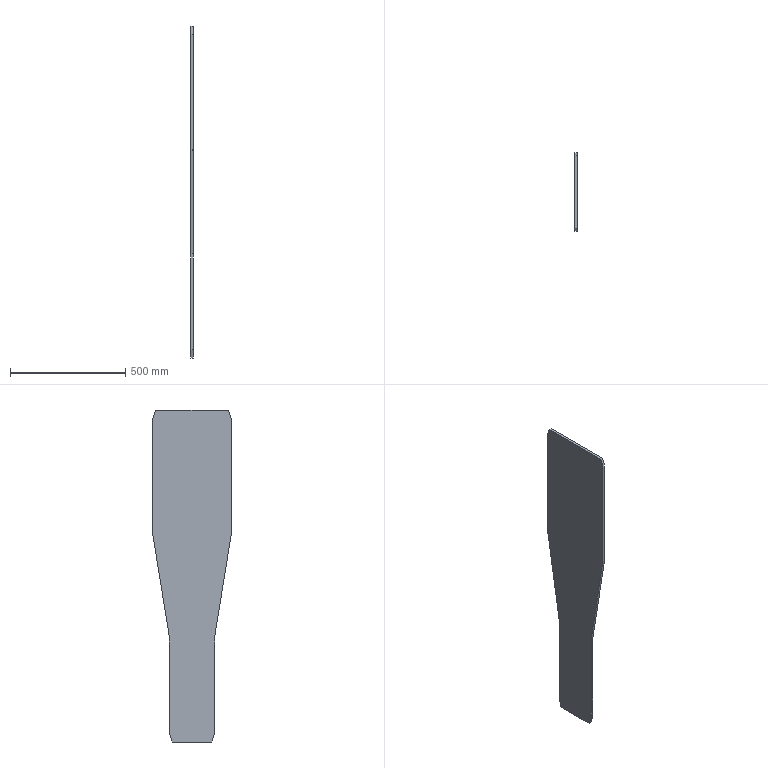Part | SolidWorks | features Extrusion 1 | 1 solid | 18 faces | box 10 x 340 x 1438 mm | volume 3900020 mm3 | plane 14 | cylinder 4 | commonest cylinder face diameters 20 x4
STEP:
#1=CARTESIAN_POINT('',(0.,85.5,-1438.));
#2=VERTEX_POINT('',#1);
#3=CARTESIAN_POINT('',(0.,97.5,-1403.));
#4=VERTEX_POINT('',#3);
#5=CARTESIAN_POINT('',(0.,85.5,-1438.));
#6=DIRECTION('',(0.,0.3243,0.9459));
#7=VECTOR('',#6,1000.);
#8=LINE('',#5,#7);
#9=EDGE_CURVE('',#2,#4,#8,.T.);
#10=ORIENTED_EDGE('',*,*,#9,.T.);
#11=CARTESIAN_POINT('',(10.,97.5,-1403.));
#12=VERTEX_POINT('',#11);
#13=CARTESIAN_POINT('',(10.,97.5,-1403.));
#14=DIRECTION('',(-1.,0.,0.));
#15=VECTOR('',#14,1000.);
#16=LINE('',#13,#15);
#17=EDGE_CURVE('',#12,#4,#16,.T.);
#18=ORIENTED_EDGE('',*,*,#17,.F.);
#19=CARTESIAN_POINT('',(10.,85.5,-1438.));
#20=VERTEX_POINT('',#19);
#21=CARTESIAN_POINT('',(10.,85.5,-1438.));
#22=DIRECTION('',(0.,0.3243,0.9459));
#23=VECTOR('',#22,1000.);
#24=LINE('',#21,#23);
#25=EDGE_CURVE('',#20,#12,#24,.T.);
#26=ORIENTED_EDGE('',*,*,#25,.F.);
#27=CARTESIAN_POINT('',(10.,85.5,-1438.));
#28=DIRECTION('',(-1.,0.,0.));
#29=VECTOR('',#28,1000.);
#30=LINE('',#27,#29);
#31=EDGE_CURVE('',#20,#2,#30,.T.);
#32=ORIENTED_EDGE('',*,*,#31,.T.);
#33=EDGE_LOOP('',(#10,#18,#26,#32));
#34=FACE_OUTER_BOUND('',#33,.T.);
#35=CARTESIAN_POINT('',(10.,85.5,-1438.));
#36=DIRECTION('',(0.,-0.9459,0.3243));
#37=DIRECTION('',(0.,-0.3243,-0.9459));
#38=AXIS2_PLACEMENT_3D('',#35,#36,#37);
#39=PLANE('',#38);
#40=ADVANCED_FACE('',(#34),#39,.F.);
#41=CARTESIAN_POINT('',(0.,97.5,-987.4));
#42=VERTEX_POINT('',#41);
#43=CARTESIAN_POINT('',(0.,97.5,-987.4));
#44=DIRECTION('',(0.,0.,1.));
#45=VECTOR('',#44,1000.);
#46=LINE('',#43,#45);
#47=EDGE_CURVE('',#4,#42,#46,.T.);
#48=ORIENTED_EDGE('',*,*,#47,.T.);
#49=CARTESIAN_POINT('',(10.,97.5,-987.4));
#50=VERTEX_POINT('',#49);
#51=CARTESIAN_POINT('',(10.,97.5,-987.4));
#52=DIRECTION('',(-1.,0.,0.));
#53=VECTOR('',#52,1000.);
#54=LINE('',#51,#53);
#55=EDGE_CURVE('',#50,#42,#54,.T.);
#56=ORIENTED_EDGE('',*,*,#55,.F.);
#57=CARTESIAN_POINT('',(10.,97.5,-987.4));
#58=DIRECTION('',(0.,0.,1.));
#59=VECTOR('',#58,1000.);
#60=LINE('',#57,#59);
#61=EDGE_CURVE('',#12,#50,#60,.T.);
#62=ORIENTED_EDGE('',*,*,#61,.F.);
#63=ORIENTED_EDGE('',*,*,#17,.T.);
#64=EDGE_LOOP('',(#48,#56,#62,#63));
#65=FACE_OUTER_BOUND('',#64,.T.);
#66=CARTESIAN_POINT('',(10.,97.5,-987.4));
#67=DIRECTION('',(0.,-1.,0.));
#68=DIRECTION('',(0.,0.,-1.));
#69=AXIS2_PLACEMENT_3D('',#66,#67,#68);
#70=PLANE('',#69);
#71=ADVANCED_FACE('',(#65),#70,.F.);
#72=CARTESIAN_POINT('',(0.,97.627,-985.81));
#73=VERTEX_POINT('',#72);
#74=CARTESIAN_POINT('',(0.,107.5,-987.4));
#75=DIRECTION('',(-1.,0.,0.));
#76=DIRECTION('',(0.,0.,1.));
#77=AXIS2_PLACEMENT_3D('',#74,#75,#76);
#78=CIRCLE('',#77,10.);
#79=EDGE_CURVE('',#42,#73,#78,.T.);
#80=ORIENTED_EDGE('',*,*,#79,.T.);
#81=CARTESIAN_POINT('',(10.,97.627,-985.81));
#82=VERTEX_POINT('',#81);
#83=CARTESIAN_POINT('',(10.,97.627,-985.81));
#84=DIRECTION('',(-1.,0.,0.));
#85=VECTOR('',#84,1000.);
#86=LINE('',#83,#85);
#87=EDGE_CURVE('',#82,#73,#86,.T.);
#88=ORIENTED_EDGE('',*,*,#87,.F.);
#89=CARTESIAN_POINT('',(10.,107.5,-987.4));
#90=DIRECTION('',(-1.,0.,0.));
#91=DIRECTION('',(0.,0.,1.));
#92=AXIS2_PLACEMENT_3D('',#89,#90,#91);
#93=CIRCLE('',#92,10.);
#94=EDGE_CURVE('',#50,#82,#93,.T.);
#95=ORIENTED_EDGE('',*,*,#94,.F.);
#96=ORIENTED_EDGE('',*,*,#55,.T.);
#97=EDGE_LOOP('',(#80,#88,#95,#96));
#98=FACE_OUTER_BOUND('',#97,.T.);
#99=CARTESIAN_POINT('',(10.,107.5,-987.4));
#100=DIRECTION('',(-1.,0.,0.));
#101=DIRECTION('',(0.,0.,1.));
#102=AXIS2_PLACEMENT_3D('',#99,#100,#101);
#103=CYLINDRICAL_SURFACE('',#102,10.);
#104=ADVANCED_FACE('',(#98),#103,.F.);
#105=CARTESIAN_POINT('',(0.,169.873,-537.39));
#106=VERTEX_POINT('',#105);
#107=CARTESIAN_POINT('',(0.,169.873,-537.39));
#108=DIRECTION('',(0.,0.1591,0.9873));
#109=VECTOR('',#108,1000.);
#110=LINE('',#107,#109);
#111=EDGE_CURVE('',#73,#106,#110,.T.);
#112=ORIENTED_EDGE('',*,*,#111,.T.);
#113=CARTESIAN_POINT('',(10.,169.873,-537.39));
#114=VERTEX_POINT('',#113);
#115=CARTESIAN_POINT('',(10.,169.873,-537.39));
#116=DIRECTION('',(-1.,0.,0.));
#117=VECTOR('',#116,1000.);
#118=LINE('',#115,#117);
#119=EDGE_CURVE('',#114,#106,#118,.T.);
#120=ORIENTED_EDGE('',*,*,#119,.F.);
#121=CARTESIAN_POINT('',(10.,169.873,-537.39));
#122=DIRECTION('',(0.,0.1591,0.9873));
#123=VECTOR('',#122,1000.);
#124=LINE('',#121,#123);
#125=EDGE_CURVE('',#82,#114,#124,.T.);
#126=ORIENTED_EDGE('',*,*,#125,.F.);
#127=ORIENTED_EDGE('',*,*,#87,.T.);
#128=EDGE_LOOP('',(#112,#120,#126,#127));
#129=FACE_OUTER_BOUND('',#128,.T.);
#130=CARTESIAN_POINT('',(10.,169.873,-537.39));
#131=DIRECTION('',(0.,-0.9873,0.1591));
#132=DIRECTION('',(0.,-0.1591,-0.9873));
#133=AXIS2_PLACEMENT_3D('',#130,#131,#132);
#134=PLANE('',#133);
#135=ADVANCED_FACE('',(#129),#134,.F.);
#136=CARTESIAN_POINT('',(0.,170.,-535.8));
#137=VERTEX_POINT('',#136);
#138=CARTESIAN_POINT('',(0.,160.,-535.8));
#139=DIRECTION('',(1.,0.,0.));
#140=DIRECTION('',(0.,0.,-1.));
#141=AXIS2_PLACEMENT_3D('',#138,#139,#140);
#142=CIRCLE('',#141,10.);
#143=EDGE_CURVE('',#106,#137,#142,.T.);
#144=ORIENTED_EDGE('',*,*,#143,.T.);
#145=CARTESIAN_POINT('',(10.,170.,-535.8));
#146=VERTEX_POINT('',#145);
#147=CARTESIAN_POINT('',(10.,170.,-535.8));
#148=DIRECTION('',(-1.,0.,0.));
#149=VECTOR('',#148,1000.);
#150=LINE('',#147,#149);
#151=EDGE_CURVE('',#146,#137,#150,.T.);
#152=ORIENTED_EDGE('',*,*,#151,.F.);
#153=CARTESIAN_POINT('',(10.,160.,-535.8));
#154=DIRECTION('',(1.,0.,0.));
#155=DIRECTION('',(0.,0.,-1.));
#156=AXIS2_PLACEMENT_3D('',#153,#154,#155);
#157=CIRCLE('',#156,10.);
#158=EDGE_CURVE('',#114,#146,#157,.T.);
#159=ORIENTED_EDGE('',*,*,#158,.F.);
#160=ORIENTED_EDGE('',*,*,#119,.T.);
#161=EDGE_LOOP('',(#144,#152,#159,#160));
#162=FACE_OUTER_BOUND('',#161,.T.);
#163=CARTESIAN_POINT('',(10.,160.,-535.8));
#164=DIRECTION('',(-1.,0.,0.));
#165=DIRECTION('',(0.,0.,1.));
#166=AXIS2_PLACEMENT_3D('',#163,#164,#165);
#167=CYLINDRICAL_SURFACE('',#166,10.);
#168=ADVANCED_FACE('',(#162),#167,.T.);
#169=CARTESIAN_POINT('',(0.,170.,-35.));
#170=VERTEX_POINT('',#169);
#171=CARTESIAN_POINT('',(0.,170.,-35.));
#172=DIRECTION('',(0.,0.,1.));
#173=VECTOR('',#172,1000.);
#174=LINE('',#171,#173);
#175=EDGE_CURVE('',#137,#170,#174,.T.);
#176=ORIENTED_EDGE('',*,*,#175,.T.);
#177=CARTESIAN_POINT('',(10.,170.,-35.));
#178=VERTEX_POINT('',#177);
#179=CARTESIAN_POINT('',(10.,170.,-35.));
#180=DIRECTION('',(-1.,0.,0.));
#181=VECTOR('',#180,1000.);
#182=LINE('',#179,#181);
#183=EDGE_CURVE('',#178,#170,#182,.T.);
#184=ORIENTED_EDGE('',*,*,#183,.F.);
#185=CARTESIAN_POINT('',(10.,170.,-35.));
#186=DIRECTION('',(0.,0.,1.));
#187=VECTOR('',#186,1000.);
#188=LINE('',#185,#187);
#189=EDGE_CURVE('',#146,#178,#188,.T.);
#190=ORIENTED_EDGE('',*,*,#189,.F.);
#191=ORIENTED_EDGE('',*,*,#151,.T.);
#192=EDGE_LOOP('',(#176,#184,#190,#191));
#193=FACE_OUTER_BOUND('',#192,.T.);
#194=CARTESIAN_POINT('',(10.,170.,-35.));
#195=DIRECTION('',(0.,-1.,0.));
#196=DIRECTION('',(0.,0.,-1.));
#197=AXIS2_PLACEMENT_3D('',#194,#195,#196);
#198=PLANE('',#197);
#199=ADVANCED_FACE('',(#193),#198,.F.);
#200=CARTESIAN_POINT('',(0.,158.,0.));
#201=VERTEX_POINT('',#200);
#202=CARTESIAN_POINT('',(0.,158.,0.));
#203=DIRECTION('',(0.,-0.3243,0.9459));
#204=VECTOR('',#203,1000.);
#205=LINE('',#202,#204);
#206=EDGE_CURVE('',#170,#201,#205,.T.);
#207=ORIENTED_EDGE('',*,*,#206,.T.);
#208=CARTESIAN_POINT('',(10.,158.,0.));
#209=VERTEX_POINT('',#208);
#210=CARTESIAN_POINT('',(10.,158.,0.));
#211=DIRECTION('',(-1.,0.,0.));
#212=VECTOR('',#211,1000.);
#213=LINE('',#210,#212);
#214=EDGE_CURVE('',#209,#201,#213,.T.);
#215=ORIENTED_EDGE('',*,*,#214,.F.);
#216=CARTESIAN_POINT('',(10.,158.,0.));
#217=DIRECTION('',(0.,-0.3243,0.9459));
#218=VECTOR('',#217,1000.);
#219=LINE('',#216,#218);
#220=EDGE_CURVE('',#178,#209,#219,.T.);
#221=ORIENTED_EDGE('',*,*,#220,.F.);
#222=ORIENTED_EDGE('',*,*,#183,.T.);
#223=EDGE_LOOP('',(#207,#215,#221,#222));
#224=FACE_OUTER_BOUND('',#223,.T.);
#225=CARTESIAN_POINT('',(10.,158.,0.));
#226=DIRECTION('',(0.,-0.9459,-0.3243));
#227=DIRECTION('',(0.,0.3243,-0.9459));
#228=AXIS2_PLACEMENT_3D('',#225,#226,#227);
#229=PLANE('',#228);
#230=ADVANCED_FACE('',(#224),#229,.F.);
#231=CARTESIAN_POINT('',(0.,-158.,0.));
#232=VERTEX_POINT('',#231);
#233=CARTESIAN_POINT('',(0.,-158.,0.));
#234=DIRECTION('',(0.,-1.,0.));
#235=VECTOR('',#234,1000.);
#236=LINE('',#233,#235);
#237=EDGE_CURVE('',#201,#232,#236,.T.);
#238=ORIENTED_EDGE('',*,*,#237,.T.);
#239=CARTESIAN_POINT('',(10.,-158.,0.));
#240=VERTEX_POINT('',#239);
#241=CARTESIAN_POINT('',(10.,-158.,0.));
#242=DIRECTION('',(-1.,0.,0.));
#243=VECTOR('',#242,1000.);
#244=LINE('',#241,#243);
#245=EDGE_CURVE('',#240,#232,#244,.T.);
#246=ORIENTED_EDGE('',*,*,#245,.F.);
#247=CARTESIAN_POINT('',(10.,-158.,0.));
#248=DIRECTION('',(0.,-1.,0.));
#249=VECTOR('',#248,1000.);
#250=LINE('',#247,#249);
#251=EDGE_CURVE('',#209,#240,#250,.T.);
#252=ORIENTED_EDGE('',*,*,#251,.F.);
#253=ORIENTED_EDGE('',*,*,#214,.T.);
#254=EDGE_LOOP('',(#238,#246,#252,#253));
#255=FACE_OUTER_BOUND('',#254,.T.);
#256=CARTESIAN_POINT('',(10.,-158.,0.));
#257=DIRECTION('',(0.,0.,-1.));
#258=DIRECTION('',(-1.,0.,0.));
#259=AXIS2_PLACEMENT_3D('',#256,#257,#258);
#260=PLANE('',#259);
#261=ADVANCED_FACE('',(#255),#260,.F.);
#262=CARTESIAN_POINT('',(0.,-170.,-35.));
#263=VERTEX_POINT('',#262);
#264=CARTESIAN_POINT('',(0.,-158.,0.));
#265=DIRECTION('',(0.,-0.3243,-0.9459));
#266=VECTOR('',#265,1000.);
#267=LINE('',#264,#266);
#268=EDGE_CURVE('',#232,#263,#267,.T.);
#269=ORIENTED_EDGE('',*,*,#268,.T.);
#270=CARTESIAN_POINT('',(10.,-170.,-35.));
#271=VERTEX_POINT('',#270);
#272=CARTESIAN_POINT('',(10.,-170.,-35.));
#273=DIRECTION('',(-1.,0.,0.));
#274=VECTOR('',#273,1000.);
#275=LINE('',#272,#274);
#276=EDGE_CURVE('',#271,#263,#275,.T.);
#277=ORIENTED_EDGE('',*,*,#276,.F.);
#278=CARTESIAN_POINT('',(10.,-158.,0.));
#279=DIRECTION('',(0.,-0.3243,-0.9459));
#280=VECTOR('',#279,1000.);
#281=LINE('',#278,#280);
#282=EDGE_CURVE('',#240,#271,#281,.T.);
#283=ORIENTED_EDGE('',*,*,#282,.F.);
#284=ORIENTED_EDGE('',*,*,#245,.T.);
#285=EDGE_LOOP('',(#269,#277,#283,#284));
#286=FACE_OUTER_BOUND('',#285,.T.);
#287=CARTESIAN_POINT('',(10.,-158.,0.));
#288=DIRECTION('',(0.,0.9459,-0.3243));
#289=DIRECTION('',(0.,0.3243,0.9459));
#290=AXIS2_PLACEMENT_3D('',#287,#288,#289);
#291=PLANE('',#290);
#292=ADVANCED_FACE('',(#286),#291,.F.);
#293=CARTESIAN_POINT('',(0.,-170.,-535.8));
#294=VERTEX_POINT('',#293);
#295=CARTESIAN_POINT('',(0.,-170.,-35.));
#296=DIRECTION('',(0.,0.,-1.));
#297=VECTOR('',#296,1000.);
#298=LINE('',#295,#297);
#299=EDGE_CURVE('',#263,#294,#298,.T.);
#300=ORIENTED_EDGE('',*,*,#299,.T.);
#301=CARTESIAN_POINT('',(10.,-170.,-535.8));
#302=VERTEX_POINT('',#301);
#303=CARTESIAN_POINT('',(10.,-170.,-535.8));
#304=DIRECTION('',(-1.,0.,0.));
#305=VECTOR('',#304,1000.);
#306=LINE('',#303,#305);
#307=EDGE_CURVE('',#302,#294,#306,.T.);
#308=ORIENTED_EDGE('',*,*,#307,.F.);
#309=CARTESIAN_POINT('',(10.,-170.,-35.));
#310=DIRECTION('',(0.,0.,-1.));
#311=VECTOR('',#310,1000.);
#312=LINE('',#309,#311);
#313=EDGE_CURVE('',#271,#302,#312,.T.);
#314=ORIENTED_EDGE('',*,*,#313,.F.);
#315=ORIENTED_EDGE('',*,*,#276,.T.);
#316=EDGE_LOOP('',(#300,#308,#314,#315));
#317=FACE_OUTER_BOUND('',#316,.T.);
#318=CARTESIAN_POINT('',(10.,-170.,-35.));
#319=DIRECTION('',(0.,1.,0.));
#320=DIRECTION('',(0.,0.,1.));
#321=AXIS2_PLACEMENT_3D('',#318,#319,#320);
#322=PLANE('',#321);
#323=ADVANCED_FACE('',(#317),#322,.F.);
#324=CARTESIAN_POINT('',(0.,-169.873,-537.39));
#325=VERTEX_POINT('',#324);
#326=CARTESIAN_POINT('',(0.,-160.,-535.8));
#327=DIRECTION('',(1.,0.,0.));
#328=DIRECTION('',(0.,0.,1.));
#329=AXIS2_PLACEMENT_3D('',#326,#327,#328);
#330=CIRCLE('',#329,10.);
#331=EDGE_CURVE('',#294,#325,#330,.T.);
#332=ORIENTED_EDGE('',*,*,#331,.T.);
#333=CARTESIAN_POINT('',(10.,-169.873,-537.39));
#334=VERTEX_POINT('',#333);
#335=CARTESIAN_POINT('',(10.,-169.873,-537.39));
#336=DIRECTION('',(-1.,0.,0.));
#337=VECTOR('',#336,1000.);
#338=LINE('',#335,#337);
#339=EDGE_CURVE('',#334,#325,#338,.T.);
#340=ORIENTED_EDGE('',*,*,#339,.F.);
#341=CARTESIAN_POINT('',(10.,-160.,-535.8));
#342=DIRECTION('',(1.,0.,0.));
#343=DIRECTION('',(0.,0.,1.));
#344=AXIS2_PLACEMENT_3D('',#341,#342,#343);
#345=CIRCLE('',#344,10.);
#346=EDGE_CURVE('',#302,#334,#345,.T.);
#347=ORIENTED_EDGE('',*,*,#346,.F.);
#348=ORIENTED_EDGE('',*,*,#307,.T.);
#349=EDGE_LOOP('',(#332,#340,#347,#348));
#350=FACE_OUTER_BOUND('',#349,.T.);
#351=CARTESIAN_POINT('',(10.,-160.,-535.8));
#352=DIRECTION('',(-1.,0.,0.));
#353=DIRECTION('',(0.,0.,1.));
#354=AXIS2_PLACEMENT_3D('',#351,#352,#353);
#355=CYLINDRICAL_SURFACE('',#354,10.);
#356=ADVANCED_FACE('',(#350),#355,.T.);
#357=CARTESIAN_POINT('',(0.,-97.627,-985.81));
#358=VERTEX_POINT('',#357);
#359=CARTESIAN_POINT('',(0.,-169.873,-537.39));
#360=DIRECTION('',(0.,0.1591,-0.9873));
#361=VECTOR('',#360,1000.);
#362=LINE('',#359,#361);
#363=EDGE_CURVE('',#325,#358,#362,.T.);
#364=ORIENTED_EDGE('',*,*,#363,.T.);
#365=CARTESIAN_POINT('',(10.,-97.627,-985.81));
#366=VERTEX_POINT('',#365);
#367=CARTESIAN_POINT('',(10.,-97.627,-985.81));
#368=DIRECTION('',(-1.,0.,0.));
#369=VECTOR('',#368,1000.);
#370=LINE('',#367,#369);
#371=EDGE_CURVE('',#366,#358,#370,.T.);
#372=ORIENTED_EDGE('',*,*,#371,.F.);
#373=CARTESIAN_POINT('',(10.,-169.873,-537.39));
#374=DIRECTION('',(0.,0.1591,-0.9873));
#375=VECTOR('',#374,1000.);
#376=LINE('',#373,#375);
#377=EDGE_CURVE('',#334,#366,#376,.T.);
#378=ORIENTED_EDGE('',*,*,#377,.F.);
#379=ORIENTED_EDGE('',*,*,#339,.T.);
#380=EDGE_LOOP('',(#364,#372,#378,#379));
#381=FACE_OUTER_BOUND('',#380,.T.);
#382=CARTESIAN_POINT('',(10.,-169.873,-537.39));
#383=DIRECTION('',(0.,0.9873,0.1591));
#384=DIRECTION('',(0.,-0.1591,0.9873));
#385=AXIS2_PLACEMENT_3D('',#382,#383,#384);
#386=PLANE('',#385);
#387=ADVANCED_FACE('',(#381),#386,.F.);
#388=CARTESIAN_POINT('',(0.,-97.5,-987.4));
#389=VERTEX_POINT('',#388);
#390=CARTESIAN_POINT('',(0.,-107.5,-987.4));
#391=DIRECTION('',(-1.,0.,0.));
#392=DIRECTION('',(0.,0.,-1.));
#393=AXIS2_PLACEMENT_3D('',#390,#391,#392);
#394=CIRCLE('',#393,10.);
#395=EDGE_CURVE('',#358,#389,#394,.T.);
#396=ORIENTED_EDGE('',*,*,#395,.T.);
#397=CARTESIAN_POINT('',(10.,-97.5,-987.4));
#398=VERTEX_POINT('',#397);
#399=CARTESIAN_POINT('',(10.,-97.5,-987.4));
#400=DIRECTION('',(-1.,0.,0.));
#401=VECTOR('',#400,1000.);
#402=LINE('',#399,#401);
#403=EDGE_CURVE('',#398,#389,#402,.T.);
#404=ORIENTED_EDGE('',*,*,#403,.F.);
#405=CARTESIAN_POINT('',(10.,-107.5,-987.4));
#406=DIRECTION('',(-1.,0.,0.));
#407=DIRECTION('',(0.,0.,-1.));
#408=AXIS2_PLACEMENT_3D('',#405,#406,#407);
#409=CIRCLE('',#408,10.);
#410=EDGE_CURVE('',#366,#398,#409,.T.);
#411=ORIENTED_EDGE('',*,*,#410,.F.);
#412=ORIENTED_EDGE('',*,*,#371,.T.);
#413=EDGE_LOOP('',(#396,#404,#411,#412));
#414=FACE_OUTER_BOUND('',#413,.T.);
#415=CARTESIAN_POINT('',(10.,-107.5,-987.4));
#416=DIRECTION('',(-1.,0.,0.));
#417=DIRECTION('',(0.,0.,1.));
#418=AXIS2_PLACEMENT_3D('',#415,#416,#417);
#419=CYLINDRICAL_SURFACE('',#418,10.);
#420=ADVANCED_FACE('',(#414),#419,.F.);
#421=CARTESIAN_POINT('',(0.,-97.5,-1403.));
#422=VERTEX_POINT('',#421);
#423=CARTESIAN_POINT('',(0.,-97.5,-987.4));
#424=DIRECTION('',(0.,0.,-1.));
#425=VECTOR('',#424,1000.);
#426=LINE('',#423,#425);
#427=EDGE_CURVE('',#389,#422,#426,.T.);
#428=ORIENTED_EDGE('',*,*,#427,.T.);
#429=CARTESIAN_POINT('',(10.,-97.5,-1403.));
#430=VERTEX_POINT('',#429);
#431=CARTESIAN_POINT('',(10.,-97.5,-1403.));
#432=DIRECTION('',(-1.,0.,0.));
#433=VECTOR('',#432,1000.);
#434=LINE('',#431,#433);
#435=EDGE_CURVE('',#430,#422,#434,.T.);
#436=ORIENTED_EDGE('',*,*,#435,.F.);
#437=CARTESIAN_POINT('',(10.,-97.5,-987.4));
#438=DIRECTION('',(0.,0.,-1.));
#439=VECTOR('',#438,1000.);
#440=LINE('',#437,#439);
#441=EDGE_CURVE('',#398,#430,#440,.T.);
#442=ORIENTED_EDGE('',*,*,#441,.F.);
#443=ORIENTED_EDGE('',*,*,#403,.T.);
#444=EDGE_LOOP('',(#428,#436,#442,#443));
#445=FACE_OUTER_BOUND('',#444,.T.);
#446=CARTESIAN_POINT('',(10.,-97.5,-987.4));
#447=DIRECTION('',(0.,1.,0.));
#448=DIRECTION('',(0.,0.,1.));
#449=AXIS2_PLACEMENT_3D('',#446,#447,#448);
#450=PLANE('',#449);
#451=ADVANCED_FACE('',(#445),#450,.F.);
#452=CARTESIAN_POINT('',(0.,-85.5,-1438.));
#453=VERTEX_POINT('',#452);
#454=CARTESIAN_POINT('',(0.,-85.5,-1438.));
#455=DIRECTION('',(0.,0.3243,-0.9459));
#456=VECTOR('',#455,1000.);
#457=LINE('',#454,#456);
#458=EDGE_CURVE('',#422,#453,#457,.T.);
#459=ORIENTED_EDGE('',*,*,#458,.T.);
#460=CARTESIAN_POINT('',(10.,-85.5,-1438.));
#461=VERTEX_POINT('',#460);
#462=CARTESIAN_POINT('',(10.,-85.5,-1438.));
#463=DIRECTION('',(-1.,0.,0.));
#464=VECTOR('',#463,1000.);
#465=LINE('',#462,#464);
#466=EDGE_CURVE('',#461,#453,#465,.T.);
#467=ORIENTED_EDGE('',*,*,#466,.F.);
#468=CARTESIAN_POINT('',(10.,-85.5,-1438.));
#469=DIRECTION('',(0.,0.3243,-0.9459));
#470=VECTOR('',#469,1000.);
#471=LINE('',#468,#470);
#472=EDGE_CURVE('',#430,#461,#471,.T.);
#473=ORIENTED_EDGE('',*,*,#472,.F.);
#474=ORIENTED_EDGE('',*,*,#435,.T.);
#475=EDGE_LOOP('',(#459,#467,#473,#474));
#476=FACE_OUTER_BOUND('',#475,.T.);
#477=CARTESIAN_POINT('',(10.,-85.5,-1438.));
#478=DIRECTION('',(0.,0.9459,0.3243));
#479=DIRECTION('',(0.,-0.3243,0.9459));
#480=AXIS2_PLACEMENT_3D('',#477,#478,#479);
#481=PLANE('',#480);
#482=ADVANCED_FACE('',(#476),#481,.F.);
#483=CARTESIAN_POINT('',(0.,85.5,-1438.));
#484=DIRECTION('',(0.,1.,0.));
#485=VECTOR('',#484,1000.);
#486=LINE('',#483,#485);
#487=EDGE_CURVE('',#453,#2,#486,.T.);
#488=ORIENTED_EDGE('',*,*,#487,.T.);
#489=ORIENTED_EDGE('',*,*,#31,.F.);
#490=CARTESIAN_POINT('',(10.,85.5,-1438.));
#491=DIRECTION('',(0.,1.,0.));
#492=VECTOR('',#491,1000.);
#493=LINE('',#490,#492);
#494=EDGE_CURVE('',#461,#20,#493,.T.);
#495=ORIENTED_EDGE('',*,*,#494,.F.);
#496=ORIENTED_EDGE('',*,*,#466,.T.);
#497=EDGE_LOOP('',(#488,#489,#495,#496));
#498=FACE_OUTER_BOUND('',#497,.T.);
#499=CARTESIAN_POINT('',(10.,85.5,-1438.));
#500=DIRECTION('',(0.,0.,1.));
#501=DIRECTION('',(1.,0.,0.));
#502=AXIS2_PLACEMENT_3D('',#499,#500,#501);
#503=PLANE('',#502);
#504=ADVANCED_FACE('',(#498),#503,.F.);
#505=ORIENTED_EDGE('',*,*,#25,.T.);
#506=ORIENTED_EDGE('',*,*,#61,.T.);
#507=ORIENTED_EDGE('',*,*,#94,.T.);
#508=ORIENTED_EDGE('',*,*,#125,.T.);
#509=ORIENTED_EDGE('',*,*,#158,.T.);
#510=ORIENTED_EDGE('',*,*,#189,.T.);
#511=ORIENTED_EDGE('',*,*,#220,.T.);
#512=ORIENTED_EDGE('',*,*,#251,.T.);
#513=ORIENTED_EDGE('',*,*,#282,.T.);
#514=ORIENTED_EDGE('',*,*,#313,.T.);
#515=ORIENTED_EDGE('',*,*,#346,.T.);
#516=ORIENTED_EDGE('',*,*,#377,.T.);
#517=ORIENTED_EDGE('',*,*,#410,.T.);
#518=ORIENTED_EDGE('',*,*,#441,.T.);
#519=ORIENTED_EDGE('',*,*,#472,.T.);
#520=ORIENTED_EDGE('',*,*,#494,.T.);
#521=EDGE_LOOP('',(#505,#506,#507,#508,#509,#510,#511,#512,#513,#514,#515,#516,#517,#518,#519,#520));
#522=FACE_OUTER_BOUND('',#521,.T.);
#523=CARTESIAN_POINT('',(10.,107.5,-987.4));
#524=DIRECTION('',(-1.,0.,0.));
#525=DIRECTION('',(0.,0.,1.));
#526=AXIS2_PLACEMENT_3D('',#523,#524,#525);
#527=PLANE('',#526);
#528=ADVANCED_FACE('',(#522),#527,.F.);
#529=ORIENTED_EDGE('',*,*,#9,.F.);
#530=ORIENTED_EDGE('',*,*,#487,.F.);
#531=ORIENTED_EDGE('',*,*,#458,.F.);
#532=ORIENTED_EDGE('',*,*,#427,.F.);
#533=ORIENTED_EDGE('',*,*,#395,.F.);
#534=ORIENTED_EDGE('',*,*,#363,.F.);
#535=ORIENTED_EDGE('',*,*,#331,.F.);
#536=ORIENTED_EDGE('',*,*,#299,.F.);
#537=ORIENTED_EDGE('',*,*,#268,.F.);
#538=ORIENTED_EDGE('',*,*,#237,.F.);
#539=ORIENTED_EDGE('',*,*,#206,.F.);
#540=ORIENTED_EDGE('',*,*,#175,.F.);
#541=ORIENTED_EDGE('',*,*,#143,.F.);
#542=ORIENTED_EDGE('',*,*,#111,.F.);
#543=ORIENTED_EDGE('',*,*,#79,.F.);
#544=ORIENTED_EDGE('',*,*,#47,.F.);
#545=EDGE_LOOP('',(#529,#530,#531,#532,#533,#534,#535,#536,#537,#538,#539,#540,#541,#542,#543,#544));
#546=FACE_OUTER_BOUND('',#545,.T.);
#547=CARTESIAN_POINT('',(0.,107.5,-987.4));
#548=DIRECTION('',(-1.,0.,0.));
#549=DIRECTION('',(0.,0.,1.));
#550=AXIS2_PLACEMENT_3D('',#547,#548,#549);
#551=PLANE('',#550);
#552=ADVANCED_FACE('',(#546),#551,.T.);
#553=CLOSED_SHELL('',(#40,#71,#104,#135,#168,#199,#230,#261,#292,#323,#356,#387,#420,#451,#482,#504,#528,#552));
#554=MANIFOLD_SOLID_BREP('',#553);
#555=CARTESIAN_POINT('',(0.,0.,0.));
#556=DIRECTION('',(0.,0.,1.));
#557=DIRECTION('',(1.,0.,0.));
#558=AXIS2_PLACEMENT_3D('',#555,#556,#557);
#559=(LENGTH_UNIT()NAMED_UNIT(*)SI_UNIT(.MILLI.,.METRE.));
#560=UNCERTAINTY_MEASURE_WITH_UNIT(LENGTH_MEASURE(0.00001),#559,'','');
#561=(NAMED_UNIT(*)PLANE_ANGLE_UNIT()SI_UNIT($,.RADIAN.));
#562=(NAMED_UNIT(*)SI_UNIT($,.STERADIAN.)SOLID_ANGLE_UNIT());
#563=(GEOMETRIC_REPRESENTATION_CONTEXT(3)GLOBAL_UNCERTAINTY_ASSIGNED_CONTEXT((#560))GLOBAL_UNIT_ASSIGNED_CONTEXT((#559,#561,#562))REPRESENTATION_CONTEXT('',''));
#564=ADVANCED_BREP_SHAPE_REPRESENTATION('',(#554,#558),#563);